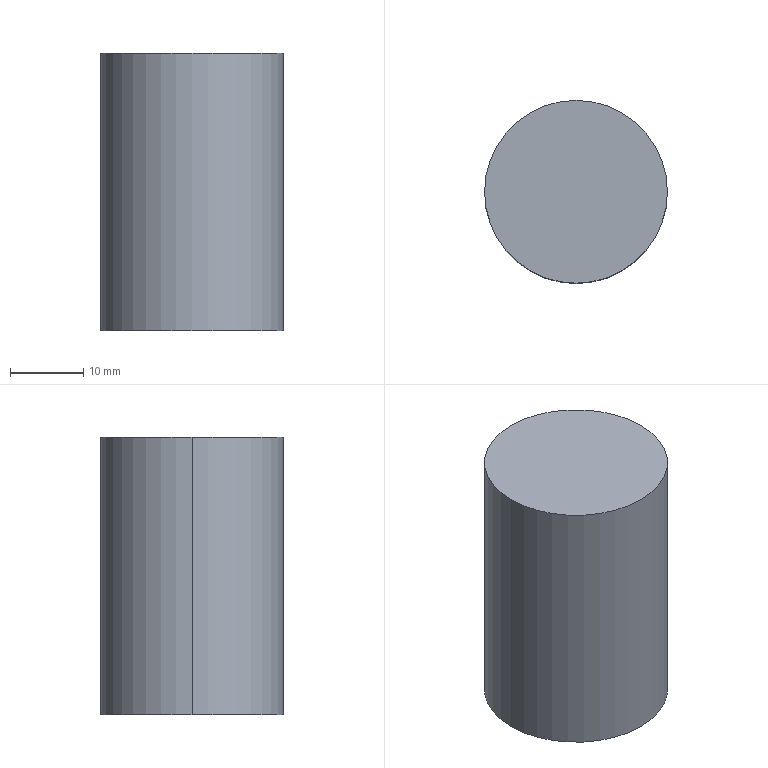Part | SolidWorks | features Extrusion 1 | 1 solid | 4 faces | box 25 x 25 x 38 mm | volume 18653 mm3 | cylinder 2 | plane 2 | commonest cylinder face diameters 25 x2
STEP:
#1=CARTESIAN_POINT('',(445.439,69.231,-33.));
#2=VERTEX_POINT('',#1);
#3=CARTESIAN_POINT('',(420.439,69.231,-33.));
#4=VERTEX_POINT('',#3);
#5=CARTESIAN_POINT('',(432.939,69.231,-33.));
#6=DIRECTION('',(0.,0.,1.));
#7=DIRECTION('',(1.,0.,0.));
#8=AXIS2_PLACEMENT_3D('',#5,#6,#7);
#9=CIRCLE('',#8,12.5);
#10=EDGE_CURVE('',#2,#4,#9,.T.);
#11=ORIENTED_EDGE('',*,*,#10,.T.);
#12=CARTESIAN_POINT('',(420.439,69.231,5.));
#13=VERTEX_POINT('',#12);
#14=CARTESIAN_POINT('',(420.439,69.231,-33.));
#15=DIRECTION('',(0.,0.,1.));
#16=VECTOR('',#15,1000.);
#17=LINE('',#14,#16);
#18=EDGE_CURVE('',#4,#13,#17,.T.);
#19=ORIENTED_EDGE('',*,*,#18,.T.);
#20=CARTESIAN_POINT('',(445.439,69.231,5.));
#21=VERTEX_POINT('',#20);
#22=CARTESIAN_POINT('',(432.939,69.231,5.));
#23=DIRECTION('',(0.,0.,1.));
#24=DIRECTION('',(1.,0.,0.));
#25=AXIS2_PLACEMENT_3D('',#22,#23,#24);
#26=CIRCLE('',#25,12.5);
#27=EDGE_CURVE('',#21,#13,#26,.T.);
#28=ORIENTED_EDGE('',*,*,#27,.F.);
#29=CARTESIAN_POINT('',(445.439,69.231,-33.));
#30=DIRECTION('',(0.,0.,1.));
#31=VECTOR('',#30,1000.);
#32=LINE('',#29,#31);
#33=EDGE_CURVE('',#2,#21,#32,.T.);
#34=ORIENTED_EDGE('',*,*,#33,.F.);
#35=EDGE_LOOP('',(#11,#19,#28,#34));
#36=FACE_OUTER_BOUND('',#35,.T.);
#37=CARTESIAN_POINT('',(432.939,69.231,-33.));
#38=DIRECTION('',(0.,0.,1.));
#39=DIRECTION('',(1.,0.,0.));
#40=AXIS2_PLACEMENT_3D('',#37,#38,#39);
#41=CYLINDRICAL_SURFACE('',#40,12.5);
#42=ADVANCED_FACE('',(#36),#41,.T.);
#43=ORIENTED_EDGE('',*,*,#18,.F.);
#44=CARTESIAN_POINT('',(432.939,69.231,-33.));
#45=DIRECTION('',(0.,0.,1.));
#46=DIRECTION('',(1.,0.,0.));
#47=AXIS2_PLACEMENT_3D('',#44,#45,#46);
#48=CIRCLE('',#47,12.5);
#49=EDGE_CURVE('',#4,#2,#48,.T.);
#50=ORIENTED_EDGE('',*,*,#49,.T.);
#51=ORIENTED_EDGE('',*,*,#33,.T.);
#52=CARTESIAN_POINT('',(432.939,69.231,5.));
#53=DIRECTION('',(0.,0.,1.));
#54=DIRECTION('',(1.,0.,0.));
#55=AXIS2_PLACEMENT_3D('',#52,#53,#54);
#56=CIRCLE('',#55,12.5);
#57=EDGE_CURVE('',#13,#21,#56,.T.);
#58=ORIENTED_EDGE('',*,*,#57,.F.);
#59=EDGE_LOOP('',(#43,#50,#51,#58));
#60=FACE_OUTER_BOUND('',#59,.T.);
#61=CARTESIAN_POINT('',(432.939,69.231,-33.));
#62=DIRECTION('',(0.,0.,1.));
#63=DIRECTION('',(1.,0.,0.));
#64=AXIS2_PLACEMENT_3D('',#61,#62,#63);
#65=CYLINDRICAL_SURFACE('',#64,12.5);
#66=ADVANCED_FACE('',(#60),#65,.T.);
#67=ORIENTED_EDGE('',*,*,#10,.F.);
#68=ORIENTED_EDGE('',*,*,#49,.F.);
#69=EDGE_LOOP('',(#67,#68));
#70=FACE_OUTER_BOUND('',#69,.T.);
#71=CARTESIAN_POINT('',(432.939,69.231,-33.));
#72=DIRECTION('',(0.,0.,1.));
#73=DIRECTION('',(1.,0.,0.));
#74=AXIS2_PLACEMENT_3D('',#71,#72,#73);
#75=PLANE('',#74);
#76=ADVANCED_FACE('',(#70),#75,.F.);
#77=ORIENTED_EDGE('',*,*,#27,.T.);
#78=ORIENTED_EDGE('',*,*,#57,.T.);
#79=EDGE_LOOP('',(#77,#78));
#80=FACE_OUTER_BOUND('',#79,.T.);
#81=CARTESIAN_POINT('',(432.939,69.231,5.));
#82=DIRECTION('',(0.,0.,1.));
#83=DIRECTION('',(1.,0.,0.));
#84=AXIS2_PLACEMENT_3D('',#81,#82,#83);
#85=PLANE('',#84);
#86=ADVANCED_FACE('',(#80),#85,.T.);
#87=CLOSED_SHELL('',(#42,#66,#76,#86));
#88=MANIFOLD_SOLID_BREP('',#87);
#89=CARTESIAN_POINT('',(0.,0.,0.));
#90=DIRECTION('',(0.,0.,1.));
#91=DIRECTION('',(1.,0.,0.));
#92=AXIS2_PLACEMENT_3D('',#89,#90,#91);
#93=(LENGTH_UNIT()NAMED_UNIT(*)SI_UNIT(.MILLI.,.METRE.));
#94=UNCERTAINTY_MEASURE_WITH_UNIT(LENGTH_MEASURE(0.00001),#93,'','');
#95=(NAMED_UNIT(*)PLANE_ANGLE_UNIT()SI_UNIT($,.RADIAN.));
#96=(NAMED_UNIT(*)SI_UNIT($,.STERADIAN.)SOLID_ANGLE_UNIT());
#97=(GEOMETRIC_REPRESENTATION_CONTEXT(3)GLOBAL_UNCERTAINTY_ASSIGNED_CONTEXT((#94))GLOBAL_UNIT_ASSIGNED_CONTEXT((#93,#95,#96))REPRESENTATION_CONTEXT('',''));
#98=ADVANCED_BREP_SHAPE_REPRESENTATION('',(#88,#92),#97);